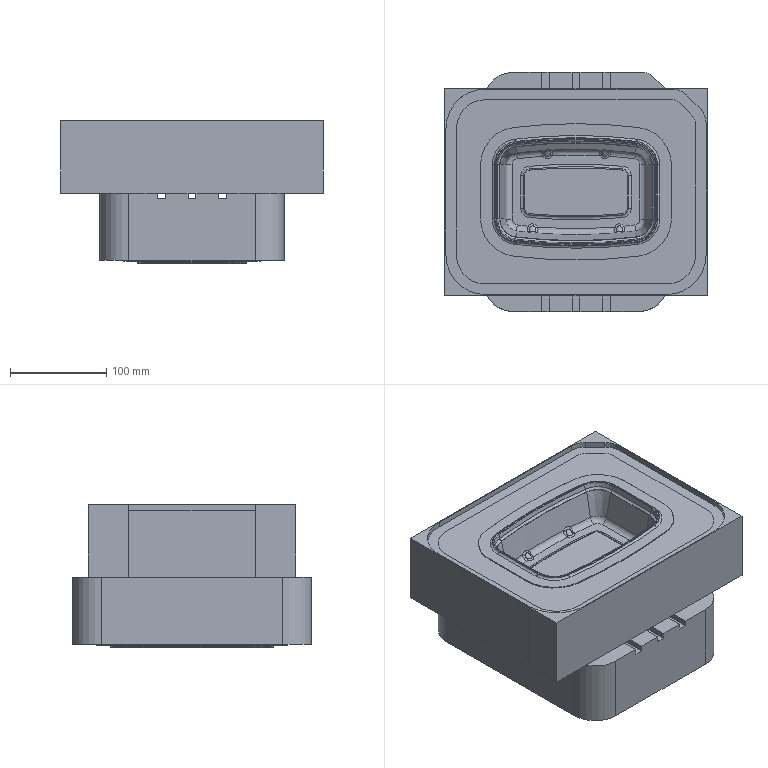NC program | NX | posted with a generic post | part box 272.387 x 248.388 x 148.5 mm
Lines 108331 to 109096 of 133013:
(FACE_MILLING_1 , TOOL : D10)
N216642 M6
N216644 G53
N216646 G17 G0 G90 X-124.08 Y85.851 S7000 M3 M8
N216648 G43 Z133. H0
N216650 Z71.707
N216652 G94 G1 X-123.652 Y86.539 Z71.665 F4000.
N216654 X-121.087 Y89.77 Z71.448
N216656 X-118.171 Y92.687 Z71.232
N216658 X-114.939 Y95.252 Z71.016
N216660 X-111.436 Y97.43 Z70.8
N216662 X-107.707 Y99.193 Z70.584
N216664 X-103.801 Y100.519 Z70.367
N216666 X-99.769 Y101.39 Z70.151
N216668 X-95.664 Y101.794 Z69.935
N216670 X-91.312 Z69.707
N216672 X100.052
N216674 G2 X111.365 Y97.107 R16.
N216676 G1 X125.507 Y82.965
N216678 G2 X130.194 Y71.651 R16.
N216680 G1 Y-65.794
N216682 G2 X94.194 Y-101.794 R36.
N216684 G1 X-94.194
N216686 G2 X-130.194 Y-65.794 R36.
N216688 G1 Y65.794
N216690 G2 X-94.194 Y101.794 R36.
N216692 G1 X-91.312
N216694 Y94.794
N216696 X100.052
N216698 G2 X106.416 Y92.157 R9.
N216700 G1 X120.558 Y78.015
N216702 G2 X123.194 Y71.651 R9.
N216704 G1 Y-65.794
N216706 G2 X94.194 Y-94.794 R29.
N216708 G1 X-94.194
N216710 G2 X-123.194 Y-65.794 R29.
N216712 G1 Y65.794
N216714 G2 X-94.194 Y94.794 R29.
N216716 G1 X-91.312
N216718 Y87.794
N216720 X100.052
N216722 G2 X101.466 Y87.208 R2.
N216724 G1 X115.608 Y73.066
N216726 G2 X116.194 Y71.651 R2.
N216728 G1 Y-65.794
N216730 G2 X94.194 Y-87.794 R22.
N216732 G1 X-94.194
N216734 G2 X-116.194 Y-65.794 R22.
N216736 G1 Y65.794
N216738 G2 X-94.194 Y87.794 R22.
N216740 G1 X-91.312
N216742 Y80.794
N216744 X97.981
N216746 X109.194 Y69.58
N216748 Y45.42
N216750 X102.194
N216752 G3 X65.81 Y73.168 R45.305
N216754 X60.501 Y73.794 R539.998
N216756 G1 X55.919 Y75.794
N216758 X38.859
N216760 G2 X55.53 Y74.331 R539.998
N216762 X55.919 Y75.794 R5.
N216764 G1 X60.501 Y73.794
N216766 X88.43
N216768 Y69.294
N216770 X93.217
N216772 X97.694 Y64.817
N216774 Y61.085
N216776 G3 X88.43 Y69.294 R49.805
N216778 G1 Y73.794
N216780 X95.081
N216782 X102.194 Y66.681
N216784 Y45.42
N216786 X104.076 Y40.307
N216788 X102.194 Y45.42
N216790 X109.194
N216792 Y-65.794
N216794 G2 X94.194 Y-80.794 R15.
N216796 G1 X60.501
N216798 Y-73.794
N216800 G3 X65.81 Y-73.168 R539.998
N216802 X102.194 Y-45.42 R45.305
N216804 G1 X104.076 Y-40.307
N216806 X102.194 Y-45.42
N216808 Y-65.794
N216810 G2 X94.194 Y-73.794 R8.
N216812 G1 X88.43
N216814 Y-69.294
N216816 G3 X97.694 Y-61.085 R49.805
N216818 G1 Y-65.794
N216820 G2 X94.194 Y-69.294 R3.5
N216822 G1 X88.43
N216824 Y-73.794
N216826 X60.501
N216828 X55.53 Y-74.331
N216830 G2 X38.859 Y-75.794 R539.998
N216832 G1 X55.919
N216834 G2 X55.53 Y-74.331 R5.
N216836 G1 X60.501 Y-73.794
N216838 Y-80.794
N216840 X-94.194
N216842 G2 X-109.194 Y-65.794 R15.
N216844 G1 Y-45.42
N216846 X-102.194
N216848 G3 X-65.81 Y-73.168 R45.305
N216850 X-60.501 Y-73.794 R539.998
N216852 G1 X-55.919 Y-75.794
N216854 X-38.859
N216856 G2 X-55.53 Y-74.331 R539.998
N216858 X-55.919 Y-75.794 R5.
N216860 G1 X-60.501 Y-73.794
N216862 X-88.43
N216864 Y-69.294
N216866 X-94.194
N216868 G2 X-97.694 Y-65.794 R3.5
N216870 G1 Y-61.085
N216872 G3 X-88.43 Y-69.294 R49.805
N216874 G1 Y-73.794
N216876 X-94.194
N216878 G2 X-102.194 Y-65.794 R8.
N216880 G1 Y-45.42
N216882 X-104.076 Y-40.307
N216884 X-102.194 Y-45.42
N216886 X-109.194
N216888 Y65.794
N216890 G2 X-94.194 Y80.794 R15.
N216892 G1 X-91.312
N216894 Y73.794
N216896 X-60.501
N216898 X-55.53 Y74.331
N216900 G2 X-38.859 Y75.794 R539.998
N216902 G1 X-55.919
N216904 G2 X-55.53 Y74.331 R5.
N216906 G1 X-60.501 Y73.794
N216908 G3 X-65.81 Y73.168 R539.998
N216910 X-102.194 Y45.42 R45.305
N216912 G1 X-104.076 Y40.307
N216914 X-102.194 Y45.42
N216916 X-100.899 Y44.888
N216918 G2 X-65.639 Y71.779 R43.906
N216920 X65.639 Y71.779 R538.598
N216922 X104.194 Y28.201 R43.906
N216924 G1 Y-28.201
N216926 G2 X65.639 Y-71.779 R43.906
N216928 X-65.639 Y-71.779 R538.598
N216930 X-104.194 Y-28.201 R43.906
N216932 G1 Y28.201
N216934 G2 X-100.899 Y44.888 R43.906
N216936 G1 X-102.194 Y45.42
N216938 Y65.794
N216940 G2 X-94.194 Y73.794 R8.
N216942 G1 X-91.312
N216944 Y69.294
N216946 X-88.43
N216948 G3 X-97.694 Y61.085 R49.805
N216950 G1 Y65.794
N216952 G2 X-94.194 Y69.294 R3.5
N216954 G1 X-91.312
N216956 G3 X-89.312 Y71.294 R2.
N216958 G1 Z70.707
N216960 G0 Z133.
(PLANAR_MILL_1 , TOOL : D10)
N216962 X70.065 Y100.794
N216964 Z70.707
N216966 G1 X100.052 Z70.681 F2000.
N216968 X101.001 Z70.68
N216970 X103.448 Y100.435 Z70.678
N216972 X105.803 Y99.679 Z70.676
N216974 X108.003 Y98.548 Z70.674
N216976 X109.987 Y97.071 Z70.671
N216978 X125.472 Y81.587 Z70.652
N216980 X126.948 Y79.603 Z70.65
N216982 X128.08 Y77.403 Z70.648
N216984 X128.835 Y75.048 Z70.646
N216986 X129.194 Y72.601 Z70.644
N216988 Y-67.243 Z70.522
N216990 X128.799 Y-71.231 Z70.518
N216992 X127.952 Y-75.148 Z70.515
N216994 X126.662 Y-78.942 Z70.511
N216996 X124.948 Y-82.564 Z70.508
N216998 X122.831 Y-85.967 Z70.504
N217000 X120.34 Y-89.106 Z70.501
N217002 X117.506 Y-91.94 Z70.497
N217004 X114.368 Y-94.431 Z70.494
N217006 X110.965 Y-96.548 Z70.49
N217008 X107.342 Y-98.262 Z70.487
N217010 X103.548 Y-99.551 Z70.483
N217012 X99.631 Y-100.399 Z70.48
N217014 X95.643 Y-100.794 Z70.476
N217016 X-95.643 Z70.309
N217018 X-99.631 Y-100.399 Z70.306
N217020 X-103.548 Y-99.551 Z70.302
N217022 X-107.342 Y-98.262 Z70.299
N217024 X-110.965 Y-96.548 Z70.295
N217026 X-114.368 Y-94.431 Z70.292
N217028 X-117.506 Y-91.94 Z70.288
N217030 X-120.34 Y-89.106 Z70.285
N217032 X-122.831 Y-85.967 Z70.281
N217034 X-124.948 Y-82.564 Z70.278
N217036 X-126.662 Y-78.942 Z70.274
N217038 X-127.952 Y-75.148 Z70.271
N217040 X-128.799 Y-71.231 Z70.267
N217042 X-129.194 Y-67.243 Z70.264
N217044 Y67.243 Z70.146
N217046 X-128.799 Y71.231 Z70.143
N217048 X-127.952 Y75.148 Z70.139
N217050 X-126.662 Y78.942 Z70.136
N217052 X-124.948 Y82.564 Z70.132
N217054 X-122.831 Y85.967 Z70.129
N217056 X-120.34 Y89.106 Z70.125
N217058 X-117.506 Y91.94 Z70.122
N217060 X-114.368 Y94.431 Z70.118
N217062 X-110.965 Y96.548 Z70.115
N217064 X-107.342 Y98.262 Z70.111
N217066 X-103.548 Y99.551 Z70.108
N217068 X-99.631 Y100.399 Z70.104
N217070 X-95.643 Y100.794 Z70.101
N217072 X101.001 Z69.929
N217074 X103.448 Y100.435 Z69.927
N217076 X105.803 Y99.679 Z69.925
N217078 X108.003 Y98.548 Z69.923
N217080 X109.987 Y97.071 Z69.921
N217082 X125.472 Y81.587 Z69.902
N217084 X126.948 Y79.603 Z69.899
N217086 X128.08 Y77.403 Z69.897
N217088 X128.835 Y75.048 Z69.895
N217090 X129.194 Y72.601 Z69.893
N217092 Y-67.243 Z69.771
N217094 X128.799 Y-71.231 Z69.767
N217096 X127.952 Y-75.148 Z69.764
N217098 X126.662 Y-78.942 Z69.76
N217100 X124.948 Y-82.564 Z69.757
N217102 X122.831 Y-85.967 Z69.753
N217104 X120.34 Y-89.106 Z69.75
N217106 X117.506 Y-91.94 Z69.746
N217108 X114.368 Y-94.431 Z69.743
N217110 X110.965 Y-96.548 Z69.739
N217112 X107.342 Y-98.262 Z69.736
N217114 X103.548 Y-99.551 Z69.732
N217116 X99.631 Y-100.399 Z69.729
N217118 X95.643 Y-100.794 Z69.725
N217120 X-95.643 Z69.559
N217122 X-99.631 Y-100.399 Z69.555
N217124 X-103.548 Y-99.551 Z69.552
N217126 X-107.342 Y-98.262 Z69.548
N217128 X-110.965 Y-96.548 Z69.545
N217130 X-114.368 Y-94.431 Z69.541
N217132 X-117.506 Y-91.94 Z69.538
N217134 X-120.34 Y-89.106 Z69.534
N217136 X-122.831 Y-85.967 Z69.531
N217138 X-124.948 Y-82.564 Z69.527
N217140 X-126.662 Y-78.942 Z69.524
N217142 X-127.952 Y-75.148 Z69.52
N217144 X-128.799 Y-71.231 Z69.517
N217146 X-129.194 Y-67.243 Z69.513
N217148 Y67.243 Z69.396
N217150 X-128.799 Y71.231 Z69.392
N217152 X-127.952 Y75.148 Z69.389
N217154 X-126.662 Y78.942 Z69.385
N217156 X-124.948 Y82.564 Z69.382
N217158 X-122.831 Y85.967 Z69.378
N217160 X-120.34 Y89.106 Z69.375
N217162 X-117.506 Y91.94 Z69.371
N217164 X-114.368 Y94.431 Z69.368
N217166 X-110.965 Y96.548 Z69.364
N217168 X-107.342 Y98.262 Z69.361
N217170 X-103.548 Y99.551 Z69.357
N217172 X-99.631 Y100.399 Z69.354
N217174 X-95.643 Y100.794 Z69.35
N217176 X101.001 Z69.179
N217178 X103.448 Y100.435 Z69.176
N217180 X105.803 Y99.679 Z69.174
N217182 X108.003 Y98.548 Z69.172
N217184 X109.987 Y97.071 Z69.17
N217186 X125.472 Y81.587 Z69.151
N217188 X126.948 Y79.603 Z69.149
N217190 X128.08 Y77.403 Z69.147
N217192 X128.835 Y75.048 Z69.144
N217194 X129.194 Y72.601 Z69.142
N217196 Y-67.243 Z69.02
N217198 X128.799 Y-71.231 Z69.017
N217200 X127.952 Y-75.148 Z69.013
N217202 X126.662 Y-78.942 Z69.01
N217204 X124.948 Y-82.564 Z69.006
N217206 X122.831 Y-85.967 Z69.003
N217208 X120.34 Y-89.106 Z68.999
N217210 X117.506 Y-91.94 Z68.996
N217212 X114.368 Y-94.431 Z68.992
N217214 X110.965 Y-96.548 Z68.989
N217216 X107.342 Y-98.262 Z68.985
N217218 X103.548 Y-99.551 Z68.982
N217220 X99.631 Y-100.399 Z68.978
N217222 X95.643 Y-100.794 Z68.975
N217224 X-95.643 Z68.808
N217226 X-99.631 Y-100.399 Z68.804
N217228 X-103.548 Y-99.551 Z68.801
N217230 X-107.342 Y-98.262 Z68.797
N217232 X-110.965 Y-96.548 Z68.794
N217234 X-114.368 Y-94.431 Z68.79
N217236 X-117.506 Y-91.94 Z68.787
N217238 X-120.34 Y-89.106 Z68.783
N217240 X-122.831 Y-85.967 Z68.78
N217242 X-124.948 Y-82.564 Z68.776
N217244 X-126.662 Y-78.942 Z68.773
N217246 X-127.952 Y-75.148 Z68.769
N217248 X-128.799 Y-71.231 Z68.766
N217250 X-129.194 Y-67.243 Z68.762
N217252 Y67.243 Z68.645
N217254 X-128.799 Y71.231 Z68.641
N217256 X-127.952 Y75.148 Z68.638
N217258 X-126.662 Y78.942 Z68.634
N217260 X-124.948 Y82.564 Z68.631
N217262 X-122.831 Y85.967 Z68.627
N217264 X-120.34 Y89.106 Z68.624
N217266 X-117.506 Y91.94 Z68.62
N217268 X-114.368 Y94.431 Z68.617
N217270 X-110.965 Y96.548 Z68.614
N217272 X-107.342 Y98.262 Z68.61
N217274 X-103.548 Y99.551 Z68.607
N217276 X-99.631 Y100.399 Z68.603
N217278 X-95.643 Y100.794 Z68.6
N217280 X101.001 Z68.428
N217282 X103.448 Y100.435 Z68.426
N217284 X105.803 Y99.679 Z68.424
N217286 X108.003 Y98.548 Z68.421
N217288 X109.987 Y97.071 Z68.419
N217290 X125.472 Y81.587 Z68.4
N217292 X126.948 Y79.603 Z68.398
N217294 X128.08 Y77.403 Z68.396
N217296 X128.835 Y75.048 Z68.394
N217298 X129.194 Y72.601 Z68.392
N217300 Y-67.243 Z68.269
N217302 X128.799 Y-71.231 Z68.266
N217304 X127.952 Y-75.148 Z68.263
N217306 X126.662 Y-78.942 Z68.259
N217308 X124.948 Y-82.564 Z68.256
N217310 X122.831 Y-85.967 Z68.252
N217312 X120.34 Y-89.106 Z68.249
N217314 X117.506 Y-91.94 Z68.245
N217316 X114.368 Y-94.431 Z68.242
N217318 X110.965 Y-96.548 Z68.238
N217320 X107.342 Y-98.262 Z68.235
N217322 X103.548 Y-99.551 Z68.231
N217324 X99.631 Y-100.399 Z68.228
N217326 X95.643 Y-100.794 Z68.224
N217328 X-95.643 Z68.057
N217330 X-99.631 Y-100.399 Z68.054
N217332 X-103.548 Y-99.551 Z68.05
N217334 X-107.342 Y-98.262 Z68.047
N217336 X-110.965 Y-96.548 Z68.043
N217338 X-114.368 Y-94.431 Z68.04
N217340 X-117.506 Y-91.94 Z68.036
N217342 X-120.34 Y-89.106 Z68.033
N217344 X-122.831 Y-85.967 Z68.029
N217346 X-124.948 Y-82.564 Z68.026
N217348 X-126.662 Y-78.942 Z68.022
N217350 X-127.952 Y-75.148 Z68.019
N217352 X-128.799 Y-71.231 Z68.015
N217354 X-129.194 Y-67.243 Z68.012
N217356 Y67.243 Z67.894
N217358 X-128.799 Y71.231 Z67.891
N217360 X-127.952 Y75.148 Z67.887
N217362 X-126.662 Y78.942 Z67.884
N217364 X-124.948 Y82.564 Z67.88
N217366 X-122.831 Y85.967 Z67.877
N217368 X-120.34 Y89.106 Z67.873
N217370 X-117.506 Y91.94 Z67.87
N217372 X-114.368 Y94.431 Z67.866
N217374 X-110.965 Y96.548 Z67.863
N217376 X-107.342 Y98.262 Z67.859
N217378 X-103.548 Y99.551 Z67.856
N217380 X-99.631 Y100.399 Z67.852
N217382 X-95.643 Y100.794 Z67.849
N217384 X101.001 Z67.677
N217386 X103.448 Y100.435 Z67.675
N217388 X105.803 Y99.679 Z67.673
N217390 X108.003 Y98.548 Z67.671
N217392 X109.987 Y97.071 Z67.669
N217394 X125.472 Y81.587 Z67.649
N217396 X126.948 Y79.603 Z67.647
N217398 X128.08 Y77.403 Z67.645
N217400 X128.835 Y75.048 Z67.643
N217402 X129.194 Y72.601 Z67.641
N217404 Y-67.243 Z67.519
N217406 X128.799 Y-71.231 Z67.515
N217408 X127.952 Y-75.148 Z67.512
N217410 X126.662 Y-78.942 Z67.508
N217412 X124.948 Y-82.564 Z67.505
N217414 X122.831 Y-85.967 Z67.501
N217416 X120.34 Y-89.106 Z67.498
N217418 X117.506 Y-91.94 Z67.494
N217420 X114.368 Y-94.431 Z67.491
N217422 X110.965 Y-96.548 Z67.487
N217424 X107.342 Y-98.262 Z67.484
N217426 X103.548 Y-99.551 Z67.48
N217428 X99.631 Y-100.399 Z67.477
N217430 X95.643 Y-100.794 Z67.473
N217432 X-95.643 Z67.306
N217434 X-99.631 Y-100.399 Z67.303
N217436 X-103.548 Y-99.551 Z67.299
N217438 X-107.342 Y-98.262 Z67.296
N217440 X-110.965 Y-96.548 Z67.292
N217442 X-114.368 Y-94.431 Z67.289
N217444 X-117.506 Y-91.94 Z67.285
N217446 X-120.34 Y-89.106 Z67.282
N217448 X-122.831 Y-85.967 Z67.278
N217450 X-124.948 Y-82.564 Z67.275
N217452 X-126.662 Y-78.942 Z67.271
N217454 X-127.952 Y-75.148 Z67.268
N217456 X-128.799 Y-71.231 Z67.264
N217458 X-129.194 Y-67.243 Z67.261
N217460 Y67.243 Z67.144
N217462 X-128.799 Y71.231 Z67.14
N217464 X-127.952 Y75.148 Z67.137
N217466 X-126.662 Y78.942 Z67.133
N217468 X-124.948 Y82.564 Z67.13
N217470 X-122.831 Y85.967 Z67.126
N217472 X-120.34 Y89.106 Z67.123
N217474 X-117.506 Y91.94 Z67.119
N217476 X-114.368 Y94.431 Z67.116
N217478 X-110.965 Y96.548 Z67.112
N217480 X-107.342 Y98.262 Z67.109
N217482 X-103.548 Y99.551 Z67.105
N217484 X-99.631 Y100.399 Z67.102
N217486 X-95.643 Y100.794 Z67.098
N217488 X101.001 Z66.927
N217490 X103.448 Y100.435 Z66.924
N217492 X105.803 Y99.679 Z66.922
N217494 X108.003 Y98.548 Z66.92
N217496 X109.987 Y97.071 Z66.918
N217498 X125.472 Y81.587 Z66.899
N217500 X126.948 Y79.603 Z66.897
N217502 X128.08 Y77.403 Z66.894
N217504 X128.835 Y75.048 Z66.892
N217506 X129.194 Y72.601 Z66.89
N217508 Y-67.243 Z66.768
N217510 X128.799 Y-71.231 Z66.765
N217512 X127.952 Y-75.148 Z66.761
N217514 X126.662 Y-78.942 Z66.758
N217516 X124.948 Y-82.564 Z66.754
N217518 X122.831 Y-85.967 Z66.751
N217520 X120.34 Y-89.106 Z66.747
N217522 X117.506 Y-91.94 Z66.744
N217524 X114.368 Y-94.431 Z66.74
N217526 X110.965 Y-96.548 Z66.737
N217528 X107.342 Y-98.262 Z66.733
N217530 X103.548 Y-99.551 Z66.73
N217532 X99.631 Y-100.399 Z66.726
N217534 X95.643 Y-100.794 Z66.723
N217536 X-95.643 Z66.556
N217538 X-99.631 Y-100.399 Z66.552
N217540 X-103.548 Y-99.551 Z66.549
N217542 X-107.342 Y-98.262 Z66.545
N217544 X-110.965 Y-96.548 Z66.542
N217546 X-114.368 Y-94.431 Z66.538
N217548 X-117.506 Y-91.94 Z66.535
N217550 X-120.34 Y-89.106 Z66.531
N217552 X-122.831 Y-85.967 Z66.528
N217554 X-124.948 Y-82.564 Z66.524
N217556 X-126.662 Y-78.942 Z66.521
N217558 X-127.952 Y-75.148 Z66.517
N217560 X-128.799 Y-71.231 Z66.514
N217562 X-129.194 Y-67.243 Z66.51
N217564 Y67.243 Z66.393
N217566 X-128.799 Y71.231 Z66.389
N217568 X-127.952 Y75.148 Z66.386
N217570 X-126.662 Y78.942 Z66.382
N217572 X-124.948 Y82.564 Z66.379
N217574 X-122.831 Y85.967 Z66.375
N217576 X-120.34 Y89.106 Z66.372
N217578 X-117.506 Y91.94 Z66.368
N217580 X-114.368 Y94.431 Z66.365
N217582 X-110.965 Y96.548 Z66.361
N217584 X-107.342 Y98.262 Z66.358
N217586 X-103.548 Y99.551 Z66.354
N217588 X-99.631 Y100.399 Z66.351
N217590 X-95.643 Y100.794 Z66.347
N217592 X101.001 Z66.176
N217594 X103.448 Y100.435 Z66.174
N217596 X105.803 Y99.679 Z66.172
N217598 X108.003 Y98.548 Z66.169
N217600 X109.987 Y97.071 Z66.167
N217602 X125.472 Y81.587 Z66.148
N217604 X126.948 Y79.603 Z66.146
N217606 X128.08 Y77.403 Z66.144
N217608 X128.835 Y75.048 Z66.142
N217610 X129.194 Y72.601 Z66.139
N217612 Y-67.243 Z66.017
N217614 X128.799 Y-71.231 Z66.014
N217616 X127.952 Y-75.148 Z66.01
N217618 X126.662 Y-78.942 Z66.007
N217620 X124.948 Y-82.564 Z66.003
N217622 X122.831 Y-85.967 Z66.
N217624 X120.34 Y-89.106 Z65.996
N217626 X117.506 Y-91.94 Z65.993
N217628 X114.368 Y-94.431 Z65.989
N217630 X110.965 Y-96.548 Z65.986
N217632 X107.342 Y-98.262 Z65.982
N217634 X103.548 Y-99.551 Z65.979
N217636 X99.631 Y-100.399 Z65.975
N217638 X95.643 Y-100.794 Z65.972
N217640 X-95.643 Z65.805
N217642 X-99.631 Y-100.399 Z65.802
N217644 X-103.548 Y-99.551 Z65.798
N217646 X-107.342 Y-98.262 Z65.795
N217648 X-110.965 Y-96.548 Z65.791
N217650 X-114.368 Y-94.431 Z65.788
N217652 X-117.506 Y-91.94 Z65.784
N217654 X-120.34 Y-89.106 Z65.781
N217656 X-122.831 Y-85.967 Z65.777
N217658 X-124.948 Y-82.564 Z65.774
N217660 X-126.662 Y-78.942 Z65.77
N217662 X-127.952 Y-75.148 Z65.767
N217664 X-128.799 Y-71.231 Z65.763
N217666 X-129.194 Y-67.243 Z65.76
N217668 Y67.243 Z65.642
N217670 X-128.799 Y71.231 Z65.639
N217672 X-127.952 Y75.148 Z65.635
N217674 X-126.662 Y78.942 Z65.632
N217676 X-124.948 Y82.564 Z65.628
N217678 X-122.831 Y85.967 Z65.625
N217680 X-120.34 Y89.106 Z65.621
N217682 X-117.506 Y91.94 Z65.618
N217684 X-114.368 Y94.431 Z65.614
N217686 X-110.965 Y96.548 Z65.611
N217688 X-107.342 Y98.262 Z65.607
N217690 X-103.548 Y99.551 Z65.604
N217692 X-99.631 Y100.399 Z65.6
N217694 X-95.643 Y100.794 Z65.597
N217696 X101.001 Z65.425
N217698 X103.448 Y100.435 Z65.423
N217700 X105.803 Y99.679 Z65.421
N217702 X108.003 Y98.548 Z65.419
N217704 X109.987 Y97.071 Z65.416
N217706 X125.472 Y81.587 Z65.397
N217708 X126.948 Y79.603 Z65.395
N217710 X128.08 Y77.403 Z65.393
N217712 X128.835 Y75.048 Z65.391
N217714 X129.194 Y72.601 Z65.389
N217716 Y-67.243 Z65.267
N217718 X128.799 Y-71.231 Z65.263
N217720 X127.952 Y-75.148 Z65.26
N217722 X126.662 Y-78.942 Z65.256
N217724 X124.948 Y-82.564 Z65.253
N217726 X122.831 Y-85.967 Z65.249
N217728 X120.34 Y-89.106 Z65.246
N217730 X117.506 Y-91.94 Z65.242
N217732 X114.368 Y-94.431 Z65.239
N217734 X110.965 Y-96.548 Z65.235
N217736 X107.342 Y-98.262 Z65.232
N217738 X103.548 Y-99.551 Z65.228
N217740 X99.631 Y-100.399 Z65.225
N217742 X95.643 Y-100.794 Z65.221
N217744 X-95.643 Z65.054
N217746 X-99.631 Y-100.399 Z65.051
N217748 X-103.548 Y-99.551 Z65.047
N217750 X-107.342 Y-98.262 Z65.044
N217752 X-110.965 Y-96.548 Z65.04
N217754 X-114.368 Y-94.431 Z65.037
N217756 X-117.506 Y-91.94 Z65.033
N217758 X-120.34 Y-89.106 Z65.03
N217760 X-122.831 Y-85.967 Z65.026
N217762 X-124.948 Y-82.564 Z65.023
N217764 X-126.662 Y-78.942 Z65.019
N217766 X-127.952 Y-75.148 Z65.016
N217768 X-128.799 Y-71.231 Z65.012
N217770 X-129.194 Y-67.243 Z65.009
N217772 Y67.243 Z64.891
N217774 X-128.799 Y71.231 Z64.888
N217776 X-127.952 Y75.148 Z64.884
N217778 X-126.662 Y78.942 Z64.881
N217780 X-124.948 Y82.564 Z64.878
N217782 X-122.831 Y85.967 Z64.874
N217784 X-120.34 Y89.106 Z64.871
N217786 X-117.506 Y91.94 Z64.867
N217788 X-114.368 Y94.431 Z64.864
N217790 X-110.965 Y96.548 Z64.86
N217792 X-107.342 Y98.262 Z64.857
N217794 X-103.548 Y99.551 Z64.853
N217796 X-99.631 Y100.399 Z64.85
N217798 X-95.643 Y100.794 Z64.846
N217800 X101.001 Z64.674
N217802 X103.448 Y100.435 Z64.672
N217804 X105.803 Y99.679 Z64.67
N217806 X108.003 Y98.548 Z64.668
N217808 X109.987 Y97.071 Z64.666
N217810 X125.472 Y81.587 Z64.647
N217812 X126.948 Y79.603 Z64.645
N217814 X128.08 Y77.403 Z64.642
N217816 X128.835 Y75.048 Z64.64
N217818 X129.194 Y72.601 Z64.638
N217820 Y-67.243 Z64.516
N217822 X128.799 Y-71.231 Z64.513
N217824 X127.952 Y-75.148 Z64.509
N217826 X126.662 Y-78.942 Z64.506
N217828 X124.948 Y-82.564 Z64.502
N217830 X122.831 Y-85.967 Z64.499
N217832 X120.34 Y-89.106 Z64.495
N217834 X117.506 Y-91.94 Z64.492
N217836 X114.368 Y-94.431 Z64.488
N217838 X110.965 Y-96.548 Z64.485
N217840 X107.342 Y-98.262 Z64.481
N217842 X103.548 Y-99.551 Z64.478
N217844 X99.631 Y-100.399 Z64.474
N217846 X95.643 Y-100.794 Z64.471
N217848 X-95.643 Z64.304
N217850 X-99.631 Y-100.399 Z64.3
N217852 X-103.548 Y-99.551 Z64.297
N217854 X-107.342 Y-98.262 Z64.293
N217856 X-110.965 Y-96.548 Z64.29
N217858 X-114.368 Y-94.431 Z64.286
N217860 X-117.506 Y-91.94 Z64.283
N217862 X-120.34 Y-89.106 Z64.279
N217864 X-122.831 Y-85.967 Z64.276
N217866 X-124.948 Y-82.564 Z64.272
N217868 X-126.662 Y-78.942 Z64.269
N217870 X-127.952 Y-75.148 Z64.265
N217872 X-128.799 Y-71.231 Z64.262
N217874 X-129.194 Y-67.243 Z64.258
N217876 Y67.243 Z64.141
N217878 X-128.799 Y71.231 Z64.137
N217880 X-127.952 Y75.148 Z64.134
N217882 X-126.662 Y78.942 Z64.13
N217884 X-124.948 Y82.564 Z64.127
N217886 X-122.831 Y85.967 Z64.123
N217888 X-120.34 Y89.106 Z64.12
N217890 X-117.506 Y91.94 Z64.116
N217892 X-114.368 Y94.431 Z64.113
N217894 X-110.965 Y96.548 Z64.109
N217896 X-107.342 Y98.262 Z64.106
N217898 X-103.548 Y99.551 Z64.102
N217900 X-99.631 Y100.399 Z64.099
N217902 X-95.643 Y100.794 Z64.095
N217904 X101.001 Z63.924
N217906 X103.448 Y100.435 Z63.922
N217908 X105.803 Y99.679 Z63.919
N217910 X108.003 Y98.548 Z63.917
N217912 X109.987 Y97.071 Z63.915
N217914 X125.472 Y81.587 Z63.896
N217916 X126.948 Y79.603 Z63.894
N217918 X128.08 Y77.403 Z63.892
N217920 X128.835 Y75.048 Z63.89
N217922 X129.194 Y72.601 Z63.887
N217924 Y-67.243 Z63.765
N217926 X128.799 Y-71.231 Z63.762
N217928 X127.952 Y-75.148 Z63.758
N217930 X126.662 Y-78.942 Z63.755
N217932 X124.948 Y-82.564 Z63.751
N217934 X122.831 Y-85.967 Z63.748
N217936 X120.34 Y-89.106 Z63.744
N217938 X117.506 Y-91.94 Z63.741
N217940 X114.368 Y-94.431 Z63.737
N217942 X110.965 Y-96.548 Z63.734
N217944 X107.342 Y-98.262 Z63.73
N217946 X103.548 Y-99.551 Z63.727
N217948 X99.631 Y-100.399 Z63.723
N217950 X95.643 Y-100.794 Z63.72
N217952 X-95.643 Z63.553
N217954 X-99.631 Y-100.399 Z63.549
N217956 X-103.548 Y-99.551 Z63.546
N217958 X-107.342 Y-98.262 Z63.542
N217960 X-110.965 Y-96.548 Z63.539
N217962 X-114.368 Y-94.431 Z63.535
N217964 X-117.506 Y-91.94 Z63.532
N217966 X-120.34 Y-89.106 Z63.528
N217968 X-122.831 Y-85.967 Z63.525
N217970 X-124.948 Y-82.564 Z63.521
N217972 X-126.662 Y-78.942 Z63.518
N217974 X-127.952 Y-75.148 Z63.514
N217976 X-128.799 Y-71.231 Z63.511
N217978 X-129.194 Y-67.243 Z63.507
N217980 Y67.243 Z63.39
N217982 X-128.799 Y71.231 Z63.387
N217984 X-127.952 Y75.148 Z63.383
N217986 X-126.662 Y78.942 Z63.38
N217988 X-124.948 Y82.564 Z63.376
N217990 X-122.831 Y85.967 Z63.373
N217992 X-120.34 Y89.106 Z63.369
N217994 X-117.506 Y91.94 Z63.366
N217996 X-114.368 Y94.431 Z63.362
N217998 X-110.965 Y96.548 Z63.359
N218000 X-107.342 Y98.262 Z63.355
N218002 X-103.548 Y99.551 Z63.352
N218004 X-99.631 Y100.399 Z63.348
N218006 X-95.643 Y100.794 Z63.345
N218008 X101.001 Z63.173
N218010 X103.448 Y100.435 Z63.171
N218012 X105.803 Y99.679 Z63.169
N218014 X108.003 Y98.548 Z63.167
N218016 X109.987 Y97.071 Z63.164
N218018 X125.472 Y81.587 Z63.145
N218020 X126.948 Y79.603 Z63.143
N218022 X128.08 Y77.403 Z63.141
N218024 X128.835 Y75.048 Z63.139
N218026 X129.194 Y72.601 Z63.137
N218028 Y-67.243 Z63.015
N218030 X128.799 Y-71.231 Z63.011
N218032 X127.952 Y-75.148 Z63.008
N218034 X126.662 Y-78.942 Z63.004
N218036 X124.948 Y-82.564 Z63.001
N218038 X122.831 Y-85.967 Z62.997
N218040 X120.34 Y-89.106 Z62.994
N218042 X117.506 Y-91.94 Z62.99
N218044 X114.368 Y-94.431 Z62.987
N218046 X110.965 Y-96.548 Z62.983
N218048 X107.342 Y-98.262 Z62.98
N218050 X103.548 Y-99.551 Z62.976
N218052 X99.631 Y-100.399 Z62.973
N218054 X95.643 Y-100.794 Z62.969
N218056 X-95.643 Z62.802
N218058 X-99.631 Y-100.399 Z62.799
N218060 X-103.548 Y-99.551 Z62.795
N218062 X-107.342 Y-98.262 Z62.792
N218064 X-110.965 Y-96.548 Z62.788
N218066 X-114.368 Y-94.431 Z62.785
N218068 X-117.506 Y-91.94 Z62.781
N218070 X-120.34 Y-89.106 Z62.778
N218072 X-122.831 Y-85.967 Z62.774
N218074 X-124.948 Y-82.564 Z62.771
N218076 X-126.662 Y-78.942 Z62.767
N218078 X-127.952 Y-75.148 Z62.764
N218080 X-128.799 Y-71.231 Z62.76
N218082 X-129.194 Y-67.243 Z62.757
N218084 Y67.243 Z62.639
N218086 X-128.799 Y71.231 Z62.636
N218088 X-127.952 Y75.148 Z62.632
N218090 X-126.662 Y78.942 Z62.629
N218092 X-124.948 Y82.564 Z62.625
N218094 X-122.831 Y85.967 Z62.622
N218096 X-120.34 Y89.106 Z62.618
N218098 X-117.506 Y91.94 Z62.615
N218100 X-114.368 Y94.431 Z62.611
N218102 X-110.965 Y96.548 Z62.608
N218104 X-107.342 Y98.262 Z62.604
N218106 X-103.548 Y99.551 Z62.601
N218108 X-99.631 Y100.399 Z62.597
N218110 X-95.643 Y100.794 Z62.594
N218112 X101.001 Z62.422
N218114 X103.448 Y100.435 Z62.42
N218116 X105.803 Y99.679 Z62.418
N218118 X108.003 Y98.548 Z62.416
N218120 X109.987 Y97.071 Z62.414
N218122 X125.472 Y81.587 Z62.395
N218124 X126.948 Y79.603 Z62.392
N218126 X128.08 Y77.403 Z62.39
N218128 X128.835 Y75.048 Z62.388
N218130 X129.194 Y72.601 Z62.386
N218132 Y-67.243 Z62.264
N218134 X128.799 Y-71.231 Z62.26
N218136 X127.952 Y-75.148 Z62.257
N218138 X126.662 Y-78.942 Z62.253
N218140 X124.948 Y-82.564 Z62.25
N218142 X122.831 Y-85.967 Z62.246
N218144 X120.34 Y-89.106 Z62.243
N218146 X117.506 Y-91.94 Z62.239
N218148 X114.368 Y-94.431 Z62.236
N218150 X110.965 Y-96.548 Z62.232
N218152 X107.342 Y-98.262 Z62.229
N218154 X103.548 Y-99.551 Z62.225
N218156 X99.631 Y-100.399 Z62.222
N218158 X95.643 Y-100.794 Z62.218
N218160 X-95.643 Z62.052